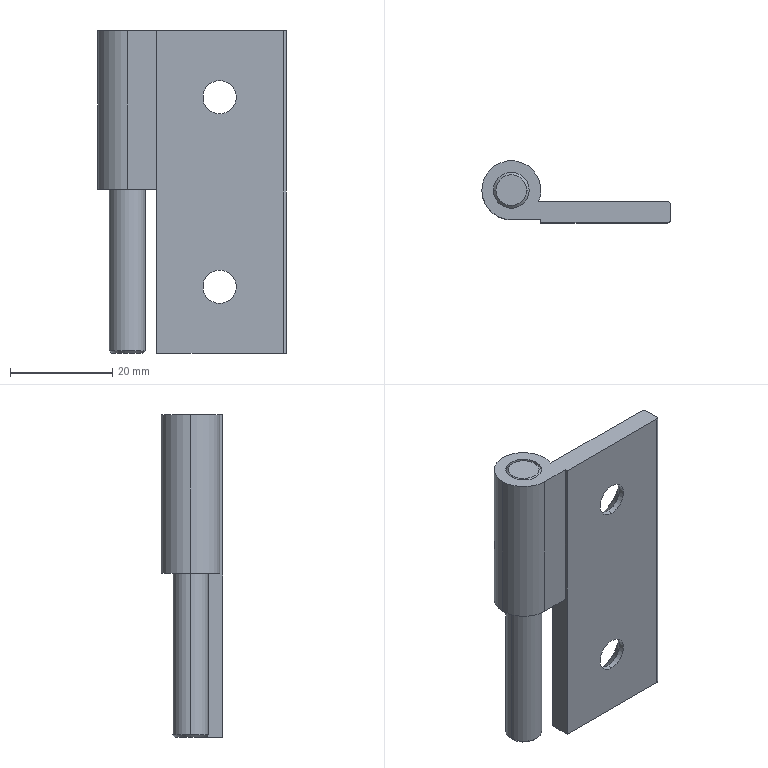Part | STEP file | Mirror _AKQ01-B-Z-R-6263-001 | 1 solid | 31 faces | box 36.75 x 12.05 x 63 mm | volume 10659 mm3 | cylinder 13 | plane 10 | cone 8 | commonest cylinder face diameters 6.5 x4 7 x4 11.5 x3 1 x2
STEP:
#1=CARTESIAN_POINT('',(18.,0.,21.75));
#2=VERTEX_POINT('',#1);
#3=CARTESIAN_POINT('',(18.,0.,15.25));
#4=VERTEX_POINT('',#3);
#5=CARTESIAN_POINT('',(18.,0.,18.5));
#6=DIRECTION('',(0.,1.,0.));
#7=DIRECTION('',(0.,0.,-1.));
#8=AXIS2_PLACEMENT_3D('',#5,#6,#7);
#9=CIRCLE('',#8,3.25);
#10=EDGE_CURVE('',#2,#4,#9,.T.);
#11=ORIENTED_EDGE('',*,*,#10,.F.);
#12=CARTESIAN_POINT('',(18.,1.1,21.75));
#13=VERTEX_POINT('',#12);
#14=CARTESIAN_POINT('',(18.,0.,21.75));
#15=DIRECTION('',(0.,1.,0.));
#16=VECTOR('',#15,1000.);
#17=LINE('',#14,#16);
#18=EDGE_CURVE('',#2,#13,#17,.T.);
#19=ORIENTED_EDGE('',*,*,#18,.T.);
#20=CARTESIAN_POINT('',(18.,1.1,15.25));
#21=VERTEX_POINT('',#20);
#22=CARTESIAN_POINT('',(18.,1.1,18.5));
#23=DIRECTION('',(0.,1.,0.));
#24=DIRECTION('',(0.,0.,-1.));
#25=AXIS2_PLACEMENT_3D('',#22,#23,#24);
#26=CIRCLE('',#25,3.25);
#27=EDGE_CURVE('',#13,#21,#26,.T.);
#28=ORIENTED_EDGE('',*,*,#27,.T.);
#29=CARTESIAN_POINT('',(18.,0.,15.25));
#30=DIRECTION('',(0.,1.,0.));
#31=VECTOR('',#30,1000.);
#32=LINE('',#29,#31);
#33=EDGE_CURVE('',#4,#21,#32,.T.);
#34=ORIENTED_EDGE('',*,*,#33,.F.);
#35=EDGE_LOOP('',(#11,#19,#28,#34));
#36=FACE_OUTER_BOUND('',#35,.T.);
#37=CARTESIAN_POINT('',(18.,0.,18.5));
#38=DIRECTION('',(0.,1.,0.));
#39=DIRECTION('',(0.,0.,-1.));
#40=AXIS2_PLACEMENT_3D('',#37,#38,#39);
#41=CYLINDRICAL_SURFACE('',#40,3.25);
#42=ADVANCED_FACE('',(#36),#41,.F.);
#43=CARTESIAN_POINT('',(18.,0.,-15.25));
#44=VERTEX_POINT('',#43);
#45=CARTESIAN_POINT('',(18.,0.,-21.75));
#46=VERTEX_POINT('',#45);
#47=CARTESIAN_POINT('',(18.,0.,-18.5));
#48=DIRECTION('',(0.,1.,0.));
#49=DIRECTION('',(0.,0.,-1.));
#50=AXIS2_PLACEMENT_3D('',#47,#48,#49);
#51=CIRCLE('',#50,3.25);
#52=EDGE_CURVE('',#44,#46,#51,.T.);
#53=ORIENTED_EDGE('',*,*,#52,.F.);
#54=CARTESIAN_POINT('',(18.,1.1,-15.25));
#55=VERTEX_POINT('',#54);
#56=CARTESIAN_POINT('',(18.,0.,-15.25));
#57=DIRECTION('',(0.,1.,0.));
#58=VECTOR('',#57,1000.);
#59=LINE('',#56,#58);
#60=EDGE_CURVE('',#44,#55,#59,.T.);
#61=ORIENTED_EDGE('',*,*,#60,.T.);
#62=CARTESIAN_POINT('',(18.,1.1,-21.75));
#63=VERTEX_POINT('',#62);
#64=CARTESIAN_POINT('',(18.,1.1,-18.5));
#65=DIRECTION('',(0.,1.,0.));
#66=DIRECTION('',(0.,0.,-1.));
#67=AXIS2_PLACEMENT_3D('',#64,#65,#66);
#68=CIRCLE('',#67,3.25);
#69=EDGE_CURVE('',#55,#63,#68,.T.);
#70=ORIENTED_EDGE('',*,*,#69,.T.);
#71=CARTESIAN_POINT('',(18.,0.,-21.75));
#72=DIRECTION('',(0.,1.,0.));
#73=VECTOR('',#72,1000.);
#74=LINE('',#71,#73);
#75=EDGE_CURVE('',#46,#63,#74,.T.);
#76=ORIENTED_EDGE('',*,*,#75,.F.);
#77=EDGE_LOOP('',(#53,#61,#70,#76));
#78=FACE_OUTER_BOUND('',#77,.T.);
#79=CARTESIAN_POINT('',(18.,0.,-18.5));
#80=DIRECTION('',(0.,1.,0.));
#81=DIRECTION('',(0.,0.,-1.));
#82=AXIS2_PLACEMENT_3D('',#79,#80,#81);
#83=CYLINDRICAL_SURFACE('',#82,3.25);
#84=ADVANCED_FACE('',(#78),#83,.F.);
#85=CARTESIAN_POINT('',(-5.75,6.3,31.5));
#86=VERTEX_POINT('',#85);
#87=CARTESIAN_POINT('',(0.,0.55,31.5));
#88=VERTEX_POINT('',#87);
#89=CARTESIAN_POINT('',(0.,6.3,31.5));
#90=DIRECTION('',(0.,0.,1.));
#91=DIRECTION('',(1.,0.,0.));
#92=AXIS2_PLACEMENT_3D('',#89,#90,#91);
#93=CIRCLE('',#92,5.75);
#94=EDGE_CURVE('',#86,#88,#93,.T.);
#95=ORIENTED_EDGE('',*,*,#94,.F.);
#96=CARTESIAN_POINT('',(-5.75,6.3,0.5));
#97=VERTEX_POINT('',#96);
#98=CARTESIAN_POINT('',(-5.75,6.3,-31.5));
#99=DIRECTION('',(0.,0.,-1.));
#100=VECTOR('',#99,1000.);
#101=LINE('',#98,#100);
#102=EDGE_CURVE('',#86,#97,#101,.T.);
#103=ORIENTED_EDGE('',*,*,#102,.T.);
#104=CARTESIAN_POINT('',(0.,0.55,0.5));
#105=VERTEX_POINT('',#104);
#106=CARTESIAN_POINT('',(0.,6.3,0.5));
#107=DIRECTION('',(0.,0.,-1.));
#108=DIRECTION('',(1.,0.,0.));
#109=AXIS2_PLACEMENT_3D('',#106,#107,#108);
#110=CIRCLE('',#109,5.75);
#111=EDGE_CURVE('',#105,#97,#110,.T.);
#112=ORIENTED_EDGE('',*,*,#111,.F.);
#113=CARTESIAN_POINT('',(0.,0.55,-31.5));
#114=DIRECTION('',(0.,0.,-1.));
#115=VECTOR('',#114,1000.);
#116=LINE('',#113,#115);
#117=EDGE_CURVE('',#88,#105,#116,.T.);
#118=ORIENTED_EDGE('',*,*,#117,.F.);
#119=EDGE_LOOP('',(#95,#103,#112,#118));
#120=FACE_OUTER_BOUND('',#119,.T.);
#121=CARTESIAN_POINT('',(0.,6.3,-31.5));
#122=DIRECTION('',(0.,0.,-1.));
#123=DIRECTION('',(1.,0.,0.));
#124=AXIS2_PLACEMENT_3D('',#121,#122,#123);
#125=CYLINDRICAL_SURFACE('',#124,5.75);
#126=ADVANCED_FACE('',(#120),#125,.T.);
#127=ORIENTED_EDGE('',*,*,#102,.F.);
#128=CARTESIAN_POINT('',(5.75,6.3,31.5));
#129=VERTEX_POINT('',#128);
#130=CARTESIAN_POINT('',(0.,6.3,31.5));
#131=DIRECTION('',(0.,0.,1.));
#132=DIRECTION('',(1.,0.,0.));
#133=AXIS2_PLACEMENT_3D('',#130,#131,#132);
#134=CIRCLE('',#133,5.75);
#135=EDGE_CURVE('',#129,#86,#134,.T.);
#136=ORIENTED_EDGE('',*,*,#135,.F.);
#137=CARTESIAN_POINT('',(5.75,6.3,0.5));
#138=VERTEX_POINT('',#137);
#139=CARTESIAN_POINT('',(5.75,6.3,-31.5));
#140=DIRECTION('',(0.,0.,-1.));
#141=VECTOR('',#140,1000.);
#142=LINE('',#139,#141);
#143=EDGE_CURVE('',#129,#138,#142,.T.);
#144=ORIENTED_EDGE('',*,*,#143,.T.);
#145=CARTESIAN_POINT('',(0.,6.3,0.5));
#146=DIRECTION('',(0.,0.,-1.));
#147=DIRECTION('',(1.,0.,0.));
#148=AXIS2_PLACEMENT_3D('',#145,#146,#147);
#149=CIRCLE('',#148,5.75);
#150=EDGE_CURVE('',#97,#138,#149,.T.);
#151=ORIENTED_EDGE('',*,*,#150,.F.);
#152=EDGE_LOOP('',(#127,#136,#144,#151));
#153=FACE_OUTER_BOUND('',#152,.T.);
#154=CARTESIAN_POINT('',(0.,6.3,-31.5));
#155=DIRECTION('',(0.,0.,-1.));
#156=DIRECTION('',(1.,0.,0.));
#157=AXIS2_PLACEMENT_3D('',#154,#155,#156);
#158=CYLINDRICAL_SURFACE('',#157,5.75);
#159=ADVANCED_FACE('',(#153),#158,.T.);
#160=CARTESIAN_POINT('',(-3.5,6.3,31.5));
#161=VERTEX_POINT('',#160);
#162=CARTESIAN_POINT('',(3.5,6.3,31.5));
#163=VERTEX_POINT('',#162);
#164=CARTESIAN_POINT('',(0.,6.3,31.5));
#165=DIRECTION('',(0.,0.,-1.));
#166=DIRECTION('',(1.,0.,0.));
#167=AXIS2_PLACEMENT_3D('',#164,#165,#166);
#168=CIRCLE('',#167,3.5);
#169=EDGE_CURVE('',#161,#163,#168,.T.);
#170=ORIENTED_EDGE('',*,*,#169,.F.);
#171=CARTESIAN_POINT('',(-3.5,6.3,31.));
#172=VERTEX_POINT('',#171);
#173=CARTESIAN_POINT('',(-3.5,6.3,-31.5));
#174=DIRECTION('',(0.,0.,-1.));
#175=VECTOR('',#174,1000.);
#176=LINE('',#173,#175);
#177=EDGE_CURVE('',#161,#172,#176,.T.);
#178=ORIENTED_EDGE('',*,*,#177,.T.);
#179=CARTESIAN_POINT('',(3.5,6.3,31.));
#180=VERTEX_POINT('',#179);
#181=CARTESIAN_POINT('',(0.,6.3,31.));
#182=DIRECTION('',(0.,0.,-1.));
#183=DIRECTION('',(1.,0.,0.));
#184=AXIS2_PLACEMENT_3D('',#181,#182,#183);
#185=CIRCLE('',#184,3.5);
#186=EDGE_CURVE('',#172,#180,#185,.T.);
#187=ORIENTED_EDGE('',*,*,#186,.T.);
#188=CARTESIAN_POINT('',(3.5,6.3,-31.5));
#189=DIRECTION('',(0.,0.,-1.));
#190=VECTOR('',#189,1000.);
#191=LINE('',#188,#190);
#192=EDGE_CURVE('',#163,#180,#191,.T.);
#193=ORIENTED_EDGE('',*,*,#192,.F.);
#194=EDGE_LOOP('',(#170,#178,#187,#193));
#195=FACE_OUTER_BOUND('',#194,.T.);
#196=CARTESIAN_POINT('',(0.,6.3,-31.5));
#197=DIRECTION('',(0.,0.,-1.));
#198=DIRECTION('',(1.,0.,0.));
#199=AXIS2_PLACEMENT_3D('',#196,#197,#198);
#200=CYLINDRICAL_SURFACE('',#199,3.5);
#201=ADVANCED_FACE('',(#195),#200,.F.);
#202=ORIENTED_EDGE('',*,*,#27,.F.);
#203=CARTESIAN_POINT('',(18.,4.1,24.75));
#204=VERTEX_POINT('',#203);
#205=CARTESIAN_POINT('',(18.,4.1,24.75));
#206=DIRECTION('',(0.,0.7071,0.7071));
#207=VECTOR('',#206,1000.);
#208=LINE('',#205,#207);
#209=EDGE_CURVE('',#13,#204,#208,.T.);
#210=ORIENTED_EDGE('',*,*,#209,.T.);
#211=CARTESIAN_POINT('',(18.,4.1,12.25));
#212=VERTEX_POINT('',#211);
#213=CARTESIAN_POINT('',(18.,4.1,18.5));
#214=DIRECTION('',(0.,-1.,0.));
#215=DIRECTION('',(0.,0.,-1.));
#216=AXIS2_PLACEMENT_3D('',#213,#214,#215);
#217=CIRCLE('',#216,6.25);
#218=EDGE_CURVE('',#212,#204,#217,.T.);
#219=ORIENTED_EDGE('',*,*,#218,.F.);
#220=CARTESIAN_POINT('',(18.,4.1,12.25));
#221=DIRECTION('',(0.,0.7071,-0.7071));
#222=VECTOR('',#221,1000.);
#223=LINE('',#220,#222);
#224=EDGE_CURVE('',#21,#212,#223,.T.);
#225=ORIENTED_EDGE('',*,*,#224,.F.);
#226=EDGE_LOOP('',(#202,#210,#219,#225));
#227=FACE_OUTER_BOUND('',#226,.T.);
#228=CARTESIAN_POINT('',(18.,4.1,18.5));
#229=DIRECTION('',(0.,1.,0.));
#230=DIRECTION('',(0.,0.,-1.));
#231=AXIS2_PLACEMENT_3D('',#228,#229,#230);
#232=CONICAL_SURFACE('',#231,6.25,0.7854);
#233=ADVANCED_FACE('',(#227),#232,.F.);
#234=ORIENTED_EDGE('',*,*,#69,.F.);
#235=CARTESIAN_POINT('',(18.,4.1,-12.25));
#236=VERTEX_POINT('',#235);
#237=CARTESIAN_POINT('',(18.,4.1,-12.25));
#238=DIRECTION('',(0.,0.7071,0.7071));
#239=VECTOR('',#238,1000.);
#240=LINE('',#237,#239);
#241=EDGE_CURVE('',#55,#236,#240,.T.);
#242=ORIENTED_EDGE('',*,*,#241,.T.);
#243=CARTESIAN_POINT('',(18.,4.1,-24.75));
#244=VERTEX_POINT('',#243);
#245=CARTESIAN_POINT('',(18.,4.1,-18.5));
#246=DIRECTION('',(0.,-1.,0.));
#247=DIRECTION('',(0.,0.,-1.));
#248=AXIS2_PLACEMENT_3D('',#245,#246,#247);
#249=CIRCLE('',#248,6.25);
#250=EDGE_CURVE('',#244,#236,#249,.T.);
#251=ORIENTED_EDGE('',*,*,#250,.F.);
#252=CARTESIAN_POINT('',(18.,4.1,-24.75));
#253=DIRECTION('',(0.,0.7071,-0.7071));
#254=VECTOR('',#253,1000.);
#255=LINE('',#252,#254);
#256=EDGE_CURVE('',#63,#244,#255,.T.);
#257=ORIENTED_EDGE('',*,*,#256,.F.);
#258=EDGE_LOOP('',(#234,#242,#251,#257));
#259=FACE_OUTER_BOUND('',#258,.T.);
#260=CARTESIAN_POINT('',(18.,4.1,-18.5));
#261=DIRECTION('',(0.,1.,0.));
#262=DIRECTION('',(0.,0.,-1.));
#263=AXIS2_PLACEMENT_3D('',#260,#261,#262);
#264=CONICAL_SURFACE('',#263,6.25,0.7854);
#265=ADVANCED_FACE('',(#259),#264,.F.);
#266=CARTESIAN_POINT('',(-3.,6.3,31.5));
#267=VERTEX_POINT('',#266);
#268=CARTESIAN_POINT('',(3.,6.3,31.5));
#269=VERTEX_POINT('',#268);
#270=CARTESIAN_POINT('',(0.,6.3,31.5));
#271=DIRECTION('',(0.,0.,1.));
#272=DIRECTION('',(1.,0.,0.));
#273=AXIS2_PLACEMENT_3D('',#270,#271,#272);
#274=CIRCLE('',#273,3.);
#275=EDGE_CURVE('',#267,#269,#274,.T.);
#276=ORIENTED_EDGE('',*,*,#275,.F.);
#277=CARTESIAN_POINT('',(-3.5,6.3,31.));
#278=DIRECTION('',(-0.7071,0.,-0.7071));
#279=VECTOR('',#278,1000.);
#280=LINE('',#277,#279);
#281=EDGE_CURVE('',#267,#172,#280,.T.);
#282=ORIENTED_EDGE('',*,*,#281,.T.);
#283=CARTESIAN_POINT('',(0.,6.3,31.));
#284=DIRECTION('',(0.,0.,-1.));
#285=DIRECTION('',(1.,0.,0.));
#286=AXIS2_PLACEMENT_3D('',#283,#284,#285);
#287=CIRCLE('',#286,3.5);
#288=EDGE_CURVE('',#180,#172,#287,.T.);
#289=ORIENTED_EDGE('',*,*,#288,.F.);
#290=CARTESIAN_POINT('',(3.5,6.3,31.));
#291=DIRECTION('',(0.7071,0.,-0.7071));
#292=VECTOR('',#291,1000.);
#293=LINE('',#290,#292);
#294=EDGE_CURVE('',#269,#180,#293,.T.);
#295=ORIENTED_EDGE('',*,*,#294,.F.);
#296=EDGE_LOOP('',(#276,#282,#289,#295));
#297=FACE_OUTER_BOUND('',#296,.T.);
#298=CARTESIAN_POINT('',(0.,6.3,31.));
#299=DIRECTION('',(0.,0.,-1.));
#300=DIRECTION('',(1.,0.,0.));
#301=AXIS2_PLACEMENT_3D('',#298,#299,#300);
#302=CONICAL_SURFACE('',#301,3.5,0.7854);
#303=ADVANCED_FACE('',(#297),#302,.T.);
#304=CARTESIAN_POINT('',(3.5,6.3,-31.));
#305=VERTEX_POINT('',#304);
#306=CARTESIAN_POINT('',(-3.5,6.3,-31.));
#307=VERTEX_POINT('',#306);
#308=CARTESIAN_POINT('',(0.,6.3,-31.));
#309=DIRECTION('',(0.,0.,-1.));
#310=DIRECTION('',(-1.,0.,0.));
#311=AXIS2_PLACEMENT_3D('',#308,#309,#310);
#312=CIRCLE('',#311,3.5);
#313=EDGE_CURVE('',#305,#307,#312,.T.);
#314=ORIENTED_EDGE('',*,*,#313,.F.);
#315=CARTESIAN_POINT('',(3.5,6.3,0.5));
#316=VERTEX_POINT('',#315);
#317=CARTESIAN_POINT('',(3.5,6.3,-31.5));
#318=DIRECTION('',(0.,0.,1.));
#319=VECTOR('',#318,1000.);
#320=LINE('',#317,#319);
#321=EDGE_CURVE('',#305,#316,#320,.T.);
#322=ORIENTED_EDGE('',*,*,#321,.T.);
#323=CARTESIAN_POINT('',(-3.5,6.3,0.5));
#324=VERTEX_POINT('',#323);
#325=CARTESIAN_POINT('',(0.,6.3,0.5));
#326=DIRECTION('',(0.,0.,-1.));
#327=DIRECTION('',(-1.,0.,0.));
#328=AXIS2_PLACEMENT_3D('',#325,#326,#327);
#329=CIRCLE('',#328,3.5);
#330=EDGE_CURVE('',#316,#324,#329,.T.);
#331=ORIENTED_EDGE('',*,*,#330,.T.);
#332=CARTESIAN_POINT('',(-3.5,6.3,-31.5));
#333=DIRECTION('',(0.,0.,1.));
#334=VECTOR('',#333,1000.);
#335=LINE('',#332,#334);
#336=EDGE_CURVE('',#307,#324,#335,.T.);
#337=ORIENTED_EDGE('',*,*,#336,.F.);
#338=EDGE_LOOP('',(#314,#322,#331,#337));
#339=FACE_OUTER_BOUND('',#338,.T.);
#340=CARTESIAN_POINT('',(0.,6.3,-31.5));
#341=DIRECTION('',(0.,0.,1.));
#342=DIRECTION('',(-1.,0.,0.));
#343=AXIS2_PLACEMENT_3D('',#340,#341,#342);
#344=CYLINDRICAL_SURFACE('',#343,3.5);
#345=ADVANCED_FACE('',(#339),#344,.T.);
#346=CARTESIAN_POINT('',(3.,6.3,-31.5));
#347=VERTEX_POINT('',#346);
#348=CARTESIAN_POINT('',(-3.,6.3,-31.5));
#349=VERTEX_POINT('',#348);
#350=CARTESIAN_POINT('',(0.,6.3,-31.5));
#351=DIRECTION('',(0.,0.,-1.));
#352=DIRECTION('',(-1.,0.,0.));
#353=AXIS2_PLACEMENT_3D('',#350,#351,#352);
#354=CIRCLE('',#353,3.);
#355=EDGE_CURVE('',#347,#349,#354,.T.);
#356=ORIENTED_EDGE('',*,*,#355,.F.);
#357=CARTESIAN_POINT('',(3.5,6.3,-31.));
#358=DIRECTION('',(0.7071,0.,0.7071));
#359=VECTOR('',#358,1000.);
#360=LINE('',#357,#359);
#361=EDGE_CURVE('',#347,#305,#360,.T.);
#362=ORIENTED_EDGE('',*,*,#361,.T.);
#363=ORIENTED_EDGE('',*,*,#313,.T.);
#364=CARTESIAN_POINT('',(-3.5,6.3,-31.));
#365=DIRECTION('',(-0.7071,0.,0.7071));
#366=VECTOR('',#365,1000.);
#367=LINE('',#364,#366);
#368=EDGE_CURVE('',#349,#307,#367,.T.);
#369=ORIENTED_EDGE('',*,*,#368,.F.);
#370=EDGE_LOOP('',(#356,#362,#363,#369));
#371=FACE_OUTER_BOUND('',#370,.T.);
#372=CARTESIAN_POINT('',(0.,6.3,-31.));
#373=DIRECTION('',(0.,0.,1.));
#374=DIRECTION('',(-1.,0.,0.));
#375=AXIS2_PLACEMENT_3D('',#372,#373,#374);
#376=CONICAL_SURFACE('',#375,3.5,0.7854);
#377=ADVANCED_FACE('',(#371),#376,.T.);
#378=CARTESIAN_POINT('',(0.,6.3,-31.5));
#379=DIRECTION('',(0.,0.,-1.));
#380=DIRECTION('',(-1.,0.,0.));
#381=AXIS2_PLACEMENT_3D('',#378,#379,#380);
#382=CIRCLE('',#381,3.);
#383=EDGE_CURVE('',#349,#347,#382,.T.);
#384=ORIENTED_EDGE('',*,*,#383,.T.);
#385=ORIENTED_EDGE('',*,*,#355,.T.);
#386=EDGE_LOOP('',(#384,#385));
#387=FACE_OUTER_BOUND('',#386,.T.);
#388=CARTESIAN_POINT('',(0.,3.3,-31.5));
#389=DIRECTION('',(0.,0.,1.));
#390=DIRECTION('',(-1.,0.,0.));
#391=AXIS2_PLACEMENT_3D('',#388,#389,#390);
#392=PLANE('',#391);
#393=ADVANCED_FACE('',(#387),#392,.F.);
#394=ORIENTED_EDGE('',*,*,#361,.F.);
#395=ORIENTED_EDGE('',*,*,#383,.F.);
#396=ORIENTED_EDGE('',*,*,#368,.T.);
#397=CARTESIAN_POINT('',(0.,6.3,-31.));
#398=DIRECTION('',(0.,0.,-1.));
#399=DIRECTION('',(-1.,0.,0.));
#400=AXIS2_PLACEMENT_3D('',#397,#398,#399);
#401=CIRCLE('',#400,3.5);
#402=EDGE_CURVE('',#307,#305,#401,.T.);
#403=ORIENTED_EDGE('',*,*,#402,.T.);
#404=EDGE_LOOP('',(#394,#395,#396,#403));
#405=FACE_OUTER_BOUND('',#404,.T.);
#406=CARTESIAN_POINT('',(0.,6.3,-31.));
#407=DIRECTION('',(0.,0.,1.));
#408=DIRECTION('',(-1.,0.,0.));
#409=AXIS2_PLACEMENT_3D('',#406,#407,#408);
#410=CONICAL_SURFACE('',#409,3.5,0.7854);
#411=ADVANCED_FACE('',(#405),#410,.T.);
#412=CARTESIAN_POINT('',(0.,6.3,31.5));
#413=DIRECTION('',(0.,0.,1.));
#414=DIRECTION('',(1.,0.,0.));
#415=AXIS2_PLACEMENT_3D('',#412,#413,#414);
#416=CIRCLE('',#415,3.);
#417=EDGE_CURVE('',#269,#267,#416,.T.);
#418=ORIENTED_EDGE('',*,*,#417,.T.);
#419=ORIENTED_EDGE('',*,*,#275,.T.);
#420=EDGE_LOOP('',(#418,#419));
#421=FACE_OUTER_BOUND('',#420,.T.);
#422=CARTESIAN_POINT('',(0.,6.3,31.5));
#423=DIRECTION('',(0.,0.,-1.));
#424=DIRECTION('',(1.,0.,0.));
#425=AXIS2_PLACEMENT_3D('',#422,#423,#424);
#426=PLANE('',#425);
#427=ADVANCED_FACE('',(#421),#426,.F.);
#428=ORIENTED_EDGE('',*,*,#321,.F.);
#429=ORIENTED_EDGE('',*,*,#402,.F.);
#430=ORIENTED_EDGE('',*,*,#336,.T.);
#431=CARTESIAN_POINT('',(0.,6.3,0.5));
#432=DIRECTION('',(0.,0.,-1.));
#433=DIRECTION('',(-1.,0.,0.));
#434=AXIS2_PLACEMENT_3D('',#431,#432,#433);
#435=CIRCLE('',#434,3.5);
#436=EDGE_CURVE('',#324,#316,#435,.T.);
#437=ORIENTED_EDGE('',*,*,#436,.T.);
#438=EDGE_LOOP('',(#428,#429,#430,#437));
#439=FACE_OUTER_BOUND('',#438,.T.);
#440=CARTESIAN_POINT('',(0.,6.3,-31.5));
#441=DIRECTION('',(0.,0.,1.));
#442=DIRECTION('',(-1.,0.,0.));
#443=AXIS2_PLACEMENT_3D('',#440,#441,#442);
#444=CYLINDRICAL_SURFACE('',#443,3.5);
#445=ADVANCED_FACE('',(#439),#444,.T.);
#446=ORIENTED_EDGE('',*,*,#281,.F.);
#447=ORIENTED_EDGE('',*,*,#417,.F.);
#448=ORIENTED_EDGE('',*,*,#294,.T.);
#449=ORIENTED_EDGE('',*,*,#186,.F.);
#450=EDGE_LOOP('',(#446,#447,#448,#449));
#451=FACE_OUTER_BOUND('',#450,.T.);
#452=CARTESIAN_POINT('',(0.,6.3,31.));
#453=DIRECTION('',(0.,0.,-1.));
#454=DIRECTION('',(1.,0.,0.));
#455=AXIS2_PLACEMENT_3D('',#452,#453,#454);
#456=CONICAL_SURFACE('',#455,3.5,0.7854);
#457=ADVANCED_FACE('',(#451),#456,.T.);
#458=CARTESIAN_POINT('',(30.5,4.1,-31.5));
#459=VERTEX_POINT('',#458);
#460=CARTESIAN_POINT('',(31.,3.6,-31.5));
#461=VERTEX_POINT('',#460);
#462=CARTESIAN_POINT('',(30.5,3.6,-31.5));
#463=DIRECTION('',(0.,0.,-1.));
#464=DIRECTION('',(1.,0.,0.));
#465=AXIS2_PLACEMENT_3D('',#462,#463,#464);
#466=CIRCLE('',#465,0.5);
#467=EDGE_CURVE('',#459,#461,#466,.T.);
#468=ORIENTED_EDGE('',*,*,#467,.F.);
#469=CARTESIAN_POINT('',(30.5,4.1,31.5));
#470=VERTEX_POINT('',#469);
#471=CARTESIAN_POINT('',(30.5,4.1,-31.5));
#472=DIRECTION('',(0.,0.,-1.));
#473=VECTOR('',#472,1000.);
#474=LINE('',#471,#473);
#475=EDGE_CURVE('',#470,#459,#474,.T.);
#476=ORIENTED_EDGE('',*,*,#475,.F.);
#477=CARTESIAN_POINT('',(31.,3.6,31.5));
#478=VERTEX_POINT('',#477);
#479=CARTESIAN_POINT('',(30.5,3.6,31.5));
#480=DIRECTION('',(0.,0.,1.));
#481=DIRECTION('',(1.,0.,0.));
#482=AXIS2_PLACEMENT_3D('',#479,#480,#481);
#483=CIRCLE('',#482,0.5);
#484=EDGE_CURVE('',#478,#470,#483,.T.);
#485=ORIENTED_EDGE('',*,*,#484,.F.);
#486=CARTESIAN_POINT('',(31.,3.6,-31.5));
#487=DIRECTION('',(0.,0.,1.));
#488=VECTOR('',#487,1000.);
#489=LINE('',#486,#488);
#490=EDGE_CURVE('',#461,#478,#489,.T.);
#491=ORIENTED_EDGE('',*,*,#490,.F.);
#492=EDGE_LOOP('',(#468,#476,#485,#491));
#493=FACE_OUTER_BOUND('',#492,.T.);
#494=CARTESIAN_POINT('',(30.5,3.6,-31.5));
#495=DIRECTION('',(0.,0.,-1.));
#496=DIRECTION('',(1.,0.,0.));
#497=AXIS2_PLACEMENT_3D('',#494,#495,#496);
#498=CYLINDRICAL_SURFACE('',#497,0.5);
#499=ADVANCED_FACE('',(#493),#498,.T.);
#500=ORIENTED_EDGE('',*,*,#241,.F.);
#501=CARTESIAN_POINT('',(18.,1.1,-18.5));
#502=DIRECTION('',(0.,1.,0.));
#503=DIRECTION('',(0.,0.,-1.));
#504=AXIS2_PLACEMENT_3D('',#501,#502,#503);
#505=CIRCLE('',#504,3.25);
#506=EDGE_CURVE('',#63,#55,#505,.T.);
#507=ORIENTED_EDGE('',*,*,#506,.F.);
#508=ORIENTED_EDGE('',*,*,#256,.T.);
#509=CARTESIAN_POINT('',(18.,4.1,-18.5));
#510=DIRECTION('',(0.,-1.,0.));
#511=DIRECTION('',(0.,0.,-1.));
#512=AXIS2_PLACEMENT_3D('',#509,#510,#511);
#513=CIRCLE('',#512,6.25);
#514=EDGE_CURVE('',#236,#244,#513,.T.);
#515=ORIENTED_EDGE('',*,*,#514,.F.);
#516=EDGE_LOOP('',(#500,#507,#508,#515));
#517=FACE_OUTER_BOUND('',#516,.T.);
#518=CARTESIAN_POINT('',(18.,4.1,-18.5));
#519=DIRECTION('',(0.,1.,0.));
#520=DIRECTION('',(0.,0.,-1.));
#521=AXIS2_PLACEMENT_3D('',#518,#519,#520);
#522=CONICAL_SURFACE('',#521,6.25,0.7854);
#523=ADVANCED_FACE('',(#517),#522,.F.);
#524=ORIENTED_EDGE('',*,*,#209,.F.);
#525=CARTESIAN_POINT('',(18.,1.1,18.5));
#526=DIRECTION('',(0.,1.,0.));
#527=DIRECTION('',(0.,0.,-1.));
#528=AXIS2_PLACEMENT_3D('',#525,#526,#527);
#529=CIRCLE('',#528,3.25);
#530=EDGE_CURVE('',#21,#13,#529,.T.);
#531=ORIENTED_EDGE('',*,*,#530,.F.);
#532=ORIENTED_EDGE('',*,*,#224,.T.);
#533=CARTESIAN_POINT('',(18.,4.1,18.5));
#534=DIRECTION('',(0.,-1.,0.));
#535=DIRECTION('',(0.,0.,-1.));
#536=AXIS2_PLACEMENT_3D('',#533,#534,#535);
#537=CIRCLE('',#536,6.25);
#538=EDGE_CURVE('',#204,#212,#537,.T.);
#539=ORIENTED_EDGE('',*,*,#538,.F.);
#540=EDGE_LOOP('',(#524,#531,#532,#539));
#541=FACE_OUTER_BOUND('',#540,.T.);
#542=CARTESIAN_POINT('',(18.,4.1,18.5));
#543=DIRECTION('',(0.,1.,0.));
#544=DIRECTION('',(0.,0.,-1.));
#545=AXIS2_PLACEMENT_3D('',#542,#543,#544);
#546=CONICAL_SURFACE('',#545,6.25,0.7854);
#547=ADVANCED_FACE('',(#541),#546,.F.);
#548=CARTESIAN_POINT('',(5.75,0.55,0.5));
#549=VERTEX_POINT('',#548);
#550=CARTESIAN_POINT('',(0.,0.55,0.5));
#551=DIRECTION('',(1.,0.,0.));
#552=VECTOR('',#551,1000.);
#553=LINE('',#550,#552);
#554=EDGE_CURVE('',#105,#549,#553,.T.);
#555=ORIENTED_EDGE('',*,*,#554,.F.);
#556=ORIENTED_EDGE('',*,*,#111,.T.);
#557=ORIENTED_EDGE('',*,*,#150,.T.);
#558=CARTESIAN_POINT('',(5.312,4.1,0.5));
#559=VERTEX_POINT('',#558);
#560=CARTESIAN_POINT('',(0.,6.3,0.5));
#561=DIRECTION('',(0.,0.,-1.));
#562=DIRECTION('',(1.,0.,0.));
#563=AXIS2_PLACEMENT_3D('',#560,#561,#562);
#564=CIRCLE('',#563,5.75);
#565=EDGE_CURVE('',#138,#559,#564,.T.);
#566=ORIENTED_EDGE('',*,*,#565,.T.);
#567=CARTESIAN_POINT('',(5.75,4.1,0.5));
#568=VERTEX_POINT('',#567);
#569=CARTESIAN_POINT('',(30.5,4.1,0.5));
#570=DIRECTION('',(-1.,0.,0.));
#571=VECTOR('',#570,1000.);
#572=LINE('',#569,#571);
#573=EDGE_CURVE('',#568,#559,#572,.T.);
#574=ORIENTED_EDGE('',*,*,#573,.F.);
#575=CARTESIAN_POINT('',(5.75,0.55,0.5));
#576=DIRECTION('',(0.,1.,0.));
#577=VECTOR('',#576,1000.);
#578=LINE('',#575,#577);
#579=EDGE_CURVE('',#549,#568,#578,.T.);
#580=ORIENTED_EDGE('',*,*,#579,.F.);
#581=EDGE_LOOP('',(#555,#556,#557,#566,#574,#580));
#582=FACE_OUTER_BOUND('',#581,.T.);
#583=ORIENTED_EDGE('',*,*,#436,.F.);
#584=ORIENTED_EDGE('',*,*,#330,.F.);
#585=EDGE_LOOP('',(#583,#584));
#586=FACE_BOUND('',#585,.T.);
#587=CARTESIAN_POINT('',(5.75,25.4,0.5));
#588=DIRECTION('',(0.,0.,-1.));
#589=DIRECTION('',(1.,0.,0.));
#590=AXIS2_PLACEMENT_3D('',#587,#588,#589);
#591=PLANE('',#590);
#592=ADVANCED_FACE('',(#582,#586),#591,.T.);
#593=ORIENTED_EDGE('',*,*,#177,.F.);
#594=CARTESIAN_POINT('',(0.,6.3,31.5));
#595=DIRECTION('',(0.,0.,-1.));
#596=DIRECTION('',(1.,0.,0.));
#597=AXIS2_PLACEMENT_3D('',#594,#595,#596);
#598=CIRCLE('',#597,3.5);
#599=EDGE_CURVE('',#163,#161,#598,.T.);
#600=ORIENTED_EDGE('',*,*,#599,.F.);
#601=ORIENTED_EDGE('',*,*,#192,.T.);
#602=ORIENTED_EDGE('',*,*,#288,.T.);
#603=EDGE_LOOP('',(#593,#600,#601,#602));
#604=FACE_OUTER_BOUND('',#603,.T.);
#605=CARTESIAN_POINT('',(0.,6.3,-31.5));
#606=DIRECTION('',(0.,0.,-1.));
#607=DIRECTION('',(1.,0.,0.));
#608=AXIS2_PLACEMENT_3D('',#605,#606,#607);
#609=CYLINDRICAL_SURFACE('',#608,3.5);
#610=ADVANCED_FACE('',(#604),#609,.F.);
#611=ORIENTED_EDGE('',*,*,#143,.F.);
#612=CARTESIAN_POINT('',(5.312,4.1,31.5));
#613=VERTEX_POINT('',#612);
#614=CARTESIAN_POINT('',(0.,6.3,31.5));
#615=DIRECTION('',(0.,0.,1.));
#616=DIRECTION('',(1.,0.,0.));
#617=AXIS2_PLACEMENT_3D('',#614,#615,#616);
#618=CIRCLE('',#617,5.75);
#619=EDGE_CURVE('',#613,#129,#618,.T.);
#620=ORIENTED_EDGE('',*,*,#619,.F.);
#621=CARTESIAN_POINT('',(5.312,4.1,-31.5));
#622=DIRECTION('',(0.,0.,1.));
#623=VECTOR('',#622,1000.);
#624=LINE('',#621,#623);
#625=EDGE_CURVE('',#559,#613,#624,.T.);
#626=ORIENTED_EDGE('',*,*,#625,.F.);
#627=ORIENTED_EDGE('',*,*,#565,.F.);
#628=EDGE_LOOP('',(#611,#620,#626,#627));
#629=FACE_OUTER_BOUND('',#628,.T.);
#630=CARTESIAN_POINT('',(0.,6.3,-31.5));
#631=DIRECTION('',(0.,0.,-1.));
#632=DIRECTION('',(1.,0.,0.));
#633=AXIS2_PLACEMENT_3D('',#630,#631,#632);
#634=CYLINDRICAL_SURFACE('',#633,5.75);
#635=ADVANCED_FACE('',(#629),#634,.T.);
#636=ORIENTED_EDGE('',*,*,#117,.T.);
#637=ORIENTED_EDGE('',*,*,#554,.T.);
#638=CARTESIAN_POINT('',(5.75,0.55,31.5));
#639=VERTEX_POINT('',#638);
#640=CARTESIAN_POINT('',(5.75,0.55,-31.5));
#641=DIRECTION('',(0.,0.,-1.));
#642=VECTOR('',#641,1000.);
#643=LINE('',#640,#642);
#644=EDGE_CURVE('',#639,#549,#643,.T.);
#645=ORIENTED_EDGE('',*,*,#644,.F.);
#646=CARTESIAN_POINT('',(0.,0.55,31.5));
#647=DIRECTION('',(1.,0.,0.));
#648=VECTOR('',#647,1000.);
#649=LINE('',#646,#648);
#650=EDGE_CURVE('',#88,#639,#649,.T.);
#651=ORIENTED_EDGE('',*,*,#650,.F.);
#652=EDGE_LOOP('',(#636,#637,#645,#651));
#653=FACE_OUTER_BOUND('',#652,.T.);
#654=CARTESIAN_POINT('',(0.,0.55,-31.5));
#655=DIRECTION('',(0.,1.,0.));
#656=DIRECTION('',(0.,0.,-1.));
#657=AXIS2_PLACEMENT_3D('',#654,#655,#656);
#658=PLANE('',#657);
#659=ADVANCED_FACE('',(#653),#658,.F.);
#660=ORIENTED_EDGE('',*,*,#490,.T.);
#661=CARTESIAN_POINT('',(31.,0.5,31.5));
#662=VERTEX_POINT('',#661);
#663=CARTESIAN_POINT('',(31.,6.3,31.5));
#664=DIRECTION('',(0.,1.,0.));
#665=VECTOR('',#664,1000.);
#666=LINE('',#663,#665);
#667=EDGE_CURVE('',#662,#478,#666,.T.);
#668=ORIENTED_EDGE('',*,*,#667,.F.);
#669=CARTESIAN_POINT('',(31.,0.5,-31.5));
#670=VERTEX_POINT('',#669);
#671=CARTESIAN_POINT('',(31.,0.5,-31.5));
#672=DIRECTION('',(0.,0.,-1.));
#673=VECTOR('',#672,1000.);
#674=LINE('',#671,#673);
#675=EDGE_CURVE('',#662,#670,#674,.T.);
#676=ORIENTED_EDGE('',*,*,#675,.T.);
#677=CARTESIAN_POINT('',(31.,6.3,-31.5));
#678=DIRECTION('',(0.,1.,0.));
#679=VECTOR('',#678,1000.);
#680=LINE('',#677,#679);
#681=EDGE_CURVE('',#670,#461,#680,.T.);
#682=ORIENTED_EDGE('',*,*,#681,.T.);
#683=EDGE_LOOP('',(#660,#668,#676,#682));
#684=FACE_OUTER_BOUND('',#683,.T.);
#685=CARTESIAN_POINT('',(31.,0.5,-31.5));
#686=DIRECTION('',(-1.,0.,0.));
#687=DIRECTION('',(0.,0.,-1.));
#688=AXIS2_PLACEMENT_3D('',#685,#686,#687);
#689=PLANE('',#688);
#690=ADVANCED_FACE('',(#684),#689,.F.);
#691=CARTESIAN_POINT('',(5.75,4.1,-31.5));
#692=VERTEX_POINT('',#691);
#693=CARTESIAN_POINT('',(0.,4.1,-31.5));
#694=DIRECTION('',(-1.,0.,0.));
#695=VECTOR('',#694,1000.);
#696=LINE('',#693,#695);
#697=EDGE_CURVE('',#459,#692,#696,.T.);
#698=ORIENTED_EDGE('',*,*,#697,.T.);
#699=CARTESIAN_POINT('',(5.75,4.1,-31.5));
#700=DIRECTION('',(0.,0.,-1.));
#701=VECTOR('',#700,1000.);
#702=LINE('',#699,#701);
#703=EDGE_CURVE('',#568,#692,#702,.T.);
#704=ORIENTED_EDGE('',*,*,#703,.F.);
#705=ORIENTED_EDGE('',*,*,#573,.T.);
#706=ORIENTED_EDGE('',*,*,#625,.T.);
#707=CARTESIAN_POINT('',(0.,4.1,31.5));
#708=DIRECTION('',(-1.,0.,0.));
#709=VECTOR('',#708,1000.);
#710=LINE('',#707,#709);
#711=EDGE_CURVE('',#470,#613,#710,.T.);
#712=ORIENTED_EDGE('',*,*,#711,.F.);
#713=ORIENTED_EDGE('',*,*,#475,.T.);
#714=EDGE_LOOP('',(#698,#704,#705,#706,#712,#713));
#715=FACE_OUTER_BOUND('',#714,.T.);
#716=ORIENTED_EDGE('',*,*,#218,.T.);
#717=ORIENTED_EDGE('',*,*,#538,.T.);
#718=EDGE_LOOP('',(#716,#717));
#719=FACE_BOUND('',#718,.T.);
#720=ORIENTED_EDGE('',*,*,#250,.T.);
#721=ORIENTED_EDGE('',*,*,#514,.T.);
#722=EDGE_LOOP('',(#720,#721));
#723=FACE_BOUND('',#722,.T.);
#724=CARTESIAN_POINT('',(30.5,4.1,-31.5));
#725=DIRECTION('',(0.,-1.,0.));
#726=DIRECTION('',(0.,0.,1.));
#727=AXIS2_PLACEMENT_3D('',#724,#725,#726);
#728=PLANE('',#727);
#729=ADVANCED_FACE('',(#715,#719,#723),#728,.F.);
#730=ORIENTED_EDGE('',*,*,#60,.F.);
#731=CARTESIAN_POINT('',(18.,0.,-18.5));
#732=DIRECTION('',(0.,1.,0.));
#733=DIRECTION('',(0.,0.,-1.));
#734=AXIS2_PLACEMENT_3D('',#731,#732,#733);
#735=CIRCLE('',#734,3.25);
#736=EDGE_CURVE('',#46,#44,#735,.T.);
#737=ORIENTED_EDGE('',*,*,#736,.F.);
#738=ORIENTED_EDGE('',*,*,#75,.T.);
#739=ORIENTED_EDGE('',*,*,#506,.T.);
#740=EDGE_LOOP('',(#730,#737,#738,#739));
#741=FACE_OUTER_BOUND('',#740,.T.);
#742=CARTESIAN_POINT('',(18.,0.,-18.5));
#743=DIRECTION('',(0.,1.,0.));
#744=DIRECTION('',(0.,0.,-1.));
#745=AXIS2_PLACEMENT_3D('',#742,#743,#744);
#746=CYLINDRICAL_SURFACE('',#745,3.25);
#747=ADVANCED_FACE('',(#741),#746,.F.);
#748=ORIENTED_EDGE('',*,*,#18,.F.);
#749=CARTESIAN_POINT('',(18.,0.,18.5));
#750=DIRECTION('',(0.,1.,0.));
#751=DIRECTION('',(0.,0.,-1.));
#752=AXIS2_PLACEMENT_3D('',#749,#750,#751);
#753=CIRCLE('',#752,3.25);
#754=EDGE_CURVE('',#4,#2,#753,.T.);
#755=ORIENTED_EDGE('',*,*,#754,.F.);
#756=ORIENTED_EDGE('',*,*,#33,.T.);
#757=ORIENTED_EDGE('',*,*,#530,.T.);
#758=EDGE_LOOP('',(#748,#755,#756,#757));
#759=FACE_OUTER_BOUND('',#758,.T.);
#760=CARTESIAN_POINT('',(18.,0.,18.5));
#761=DIRECTION('',(0.,1.,0.));
#762=DIRECTION('',(0.,0.,-1.));
#763=AXIS2_PLACEMENT_3D('',#760,#761,#762);
#764=CYLINDRICAL_SURFACE('',#763,3.25);
#765=ADVANCED_FACE('',(#759),#764,.F.);
#766=ORIENTED_EDGE('',*,*,#703,.T.);
#767=CARTESIAN_POINT('',(5.75,0.,-31.5));
#768=VERTEX_POINT('',#767);
#769=CARTESIAN_POINT('',(5.75,6.3,-31.5));
#770=DIRECTION('',(0.,-1.,0.));
#771=VECTOR('',#770,1000.);
#772=LINE('',#769,#771);
#773=EDGE_CURVE('',#692,#768,#772,.T.);
#774=ORIENTED_EDGE('',*,*,#773,.T.);
#775=CARTESIAN_POINT('',(5.75,0.,31.5));
#776=VERTEX_POINT('',#775);
#777=CARTESIAN_POINT('',(5.75,0.,-31.5));
#778=DIRECTION('',(0.,0.,-1.));
#779=VECTOR('',#778,1000.);
#780=LINE('',#777,#779);
#781=EDGE_CURVE('',#776,#768,#780,.T.);
#782=ORIENTED_EDGE('',*,*,#781,.F.);
#783=CARTESIAN_POINT('',(5.75,6.3,31.5));
#784=DIRECTION('',(0.,-1.,0.));
#785=VECTOR('',#784,1000.);
#786=LINE('',#783,#785);
#787=EDGE_CURVE('',#639,#776,#786,.T.);
#788=ORIENTED_EDGE('',*,*,#787,.F.);
#789=ORIENTED_EDGE('',*,*,#644,.T.);
#790=ORIENTED_EDGE('',*,*,#579,.T.);
#791=EDGE_LOOP('',(#766,#774,#782,#788,#789,#790));
#792=FACE_OUTER_BOUND('',#791,.T.);
#793=CARTESIAN_POINT('',(5.75,0.55,-31.5));
#794=DIRECTION('',(1.,0.,0.));
#795=DIRECTION('',(0.,1.,0.));
#796=AXIS2_PLACEMENT_3D('',#793,#794,#795);
#797=PLANE('',#796);
#798=ADVANCED_FACE('',(#792),#797,.F.);
#799=ORIENTED_EDGE('',*,*,#681,.F.);
#800=CARTESIAN_POINT('',(30.5,0.,-31.5));
#801=VERTEX_POINT('',#800);
#802=CARTESIAN_POINT('',(30.5,0.5,-31.5));
#803=DIRECTION('',(0.,0.,-1.));
#804=DIRECTION('',(1.,0.,0.));
#805=AXIS2_PLACEMENT_3D('',#802,#803,#804);
#806=CIRCLE('',#805,0.5);
#807=EDGE_CURVE('',#670,#801,#806,.T.);
#808=ORIENTED_EDGE('',*,*,#807,.T.);
#809=CARTESIAN_POINT('',(5.75,0.,-31.5));
#810=DIRECTION('',(1.,0.,0.));
#811=VECTOR('',#810,1000.);
#812=LINE('',#809,#811);
#813=EDGE_CURVE('',#768,#801,#812,.T.);
#814=ORIENTED_EDGE('',*,*,#813,.F.);
#815=ORIENTED_EDGE('',*,*,#773,.F.);
#816=ORIENTED_EDGE('',*,*,#697,.F.);
#817=ORIENTED_EDGE('',*,*,#467,.T.);
#818=EDGE_LOOP('',(#799,#808,#814,#815,#816,#817));
#819=FACE_OUTER_BOUND('',#818,.T.);
#820=CARTESIAN_POINT('',(0.,6.3,-31.5));
#821=DIRECTION('',(0.,0.,-1.));
#822=DIRECTION('',(1.,0.,0.));
#823=AXIS2_PLACEMENT_3D('',#820,#821,#822);
#824=PLANE('',#823);
#825=ADVANCED_FACE('',(#819),#824,.T.);
#826=ORIENTED_EDGE('',*,*,#807,.F.);
#827=ORIENTED_EDGE('',*,*,#675,.F.);
#828=CARTESIAN_POINT('',(30.5,0.,31.5));
#829=VERTEX_POINT('',#828);
#830=CARTESIAN_POINT('',(30.5,0.5,31.5));
#831=DIRECTION('',(0.,0.,1.));
#832=DIRECTION('',(1.,0.,0.));
#833=AXIS2_PLACEMENT_3D('',#830,#831,#832);
#834=CIRCLE('',#833,0.5);
#835=EDGE_CURVE('',#829,#662,#834,.T.);
#836=ORIENTED_EDGE('',*,*,#835,.F.);
#837=CARTESIAN_POINT('',(30.5,0.,-31.5));
#838=DIRECTION('',(0.,0.,1.));
#839=VECTOR('',#838,1000.);
#840=LINE('',#837,#839);
#841=EDGE_CURVE('',#801,#829,#840,.T.);
#842=ORIENTED_EDGE('',*,*,#841,.F.);
#843=EDGE_LOOP('',(#826,#827,#836,#842));
#844=FACE_OUTER_BOUND('',#843,.T.);
#845=CARTESIAN_POINT('',(30.5,0.5,-31.5));
#846=DIRECTION('',(0.,0.,-1.));
#847=DIRECTION('',(1.,0.,0.));
#848=AXIS2_PLACEMENT_3D('',#845,#846,#847);
#849=CYLINDRICAL_SURFACE('',#848,0.5);
#850=ADVANCED_FACE('',(#844),#849,.T.);
#851=ORIENTED_EDGE('',*,*,#484,.T.);
#852=ORIENTED_EDGE('',*,*,#711,.T.);
#853=ORIENTED_EDGE('',*,*,#619,.T.);
#854=ORIENTED_EDGE('',*,*,#135,.T.);
#855=ORIENTED_EDGE('',*,*,#94,.T.);
#856=ORIENTED_EDGE('',*,*,#650,.T.);
#857=ORIENTED_EDGE('',*,*,#787,.T.);
#858=CARTESIAN_POINT('',(5.75,0.,31.5));
#859=DIRECTION('',(-1.,0.,0.));
#860=VECTOR('',#859,1000.);
#861=LINE('',#858,#860);
#862=EDGE_CURVE('',#829,#776,#861,.T.);
#863=ORIENTED_EDGE('',*,*,#862,.F.);
#864=ORIENTED_EDGE('',*,*,#835,.T.);
#865=ORIENTED_EDGE('',*,*,#667,.T.);
#866=EDGE_LOOP('',(#851,#852,#853,#854,#855,#856,#857,#863,#864,#865));
#867=FACE_OUTER_BOUND('',#866,.T.);
#868=ORIENTED_EDGE('',*,*,#599,.T.);
#869=ORIENTED_EDGE('',*,*,#169,.T.);
#870=EDGE_LOOP('',(#868,#869));
#871=FACE_BOUND('',#870,.T.);
#872=CARTESIAN_POINT('',(0.,6.3,31.5));
#873=DIRECTION('',(0.,0.,-1.));
#874=DIRECTION('',(1.,0.,0.));
#875=AXIS2_PLACEMENT_3D('',#872,#873,#874);
#876=PLANE('',#875);
#877=ADVANCED_FACE('',(#867,#871),#876,.F.);
#878=ORIENTED_EDGE('',*,*,#841,.T.);
#879=ORIENTED_EDGE('',*,*,#862,.T.);
#880=ORIENTED_EDGE('',*,*,#781,.T.);
#881=ORIENTED_EDGE('',*,*,#813,.T.);
#882=EDGE_LOOP('',(#878,#879,#880,#881));
#883=FACE_OUTER_BOUND('',#882,.T.);
#884=ORIENTED_EDGE('',*,*,#754,.T.);
#885=ORIENTED_EDGE('',*,*,#10,.T.);
#886=EDGE_LOOP('',(#884,#885));
#887=FACE_BOUND('',#886,.T.);
#888=ORIENTED_EDGE('',*,*,#736,.T.);
#889=ORIENTED_EDGE('',*,*,#52,.T.);
#890=EDGE_LOOP('',(#888,#889));
#891=FACE_BOUND('',#890,.T.);
#892=CARTESIAN_POINT('',(5.75,0.,-31.5));
#893=DIRECTION('',(0.,1.,0.));
#894=DIRECTION('',(0.,0.,-1.));
#895=AXIS2_PLACEMENT_3D('',#892,#893,#894);
#896=PLANE('',#895);
#897=ADVANCED_FACE('',(#883,#887,#891),#896,.F.);
#898=CLOSED_SHELL('',(#42,#84,#126,#159,#201,#233,#265,#303,#345,#377,#393,#411,#427,#445,#457,#499,#523,#547,#592,#610,#635,#659,#690,#729,#747,#765,#798,#825,#850,#877,#897));
#899=MANIFOLD_SOLID_BREP('',#898);
#900=CARTESIAN_POINT('',(0.,0.,0.));
#901=DIRECTION('',(0.,0.,1.));
#902=DIRECTION('',(1.,0.,0.));
#903=AXIS2_PLACEMENT_3D('',#900,#901,#902);
#904=(LENGTH_UNIT()NAMED_UNIT(*)SI_UNIT(.MILLI.,.METRE.));
#905=UNCERTAINTY_MEASURE_WITH_UNIT(LENGTH_MEASURE(0.00001),#904,'','');
#906=(NAMED_UNIT(*)PLANE_ANGLE_UNIT()SI_UNIT($,.RADIAN.));
#907=(NAMED_UNIT(*)SI_UNIT($,.STERADIAN.)SOLID_ANGLE_UNIT());
#908=(GEOMETRIC_REPRESENTATION_CONTEXT(3)GLOBAL_UNCERTAINTY_ASSIGNED_CONTEXT((#905))GLOBAL_UNIT_ASSIGNED_CONTEXT((#904,#906,#907))REPRESENTATION_CONTEXT('',''));
#909=ADVANCED_BREP_SHAPE_REPRESENTATION('',(#899,#903),#908);